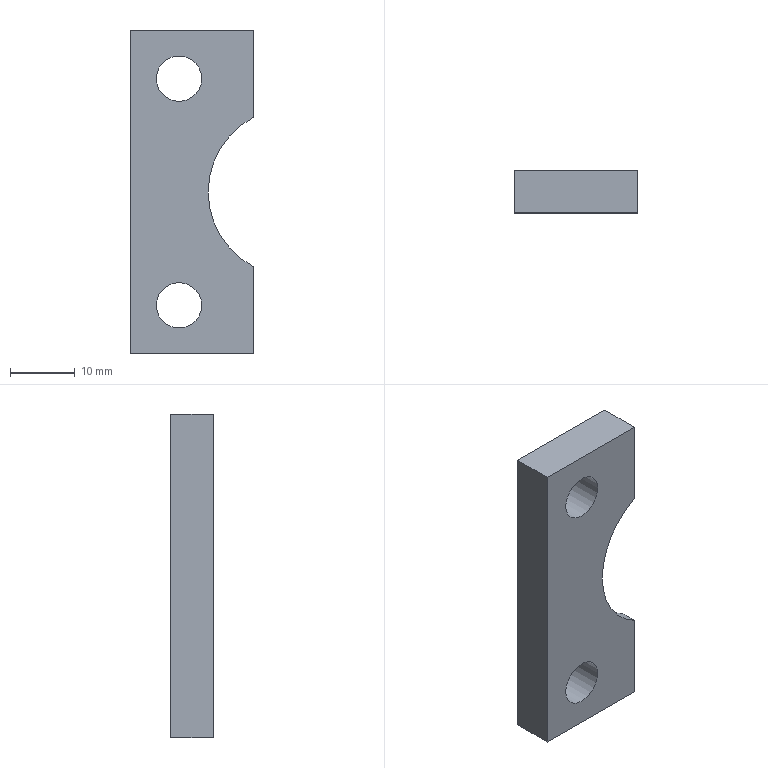Part | NX | features solid 2 | 1 solid | 12 faces | box 19 x 6.5 x 50 mm | volume 4528 mm3 | plane 8 | cylinder 4 | commonest cylinder face diameters 7 x2 26 x1 32 x1
STEP:
#1=CARTESIAN_POINT('',(694.,845.,-199.832));
#2=VERTEX_POINT('',#1);
#3=CARTESIAN_POINT('',(694.,849.,-199.832));
#4=VERTEX_POINT('',#3);
#5=CARTESIAN_POINT('',(694.,842.5,-199.832));
#6=DIRECTION('',(0.,1.,0.));
#7=VECTOR('',#6,1000.);
#8=LINE('',#5,#7);
#9=EDGE_CURVE('',#2,#4,#8,.T.);
#10=ORIENTED_EDGE('',*,*,#9,.T.);
#11=CARTESIAN_POINT('',(694.,849.,-170.168));
#12=VERTEX_POINT('',#11);
#13=CARTESIAN_POINT('',(700.,849.,-185.));
#14=DIRECTION('',(0.,1.,0.));
#15=DIRECTION('',(-1.,0.,0.));
#16=AXIS2_PLACEMENT_3D('',#13,#14,#15);
#17=CIRCLE('',#16,16.);
#18=EDGE_CURVE('',#4,#12,#17,.T.);
#19=ORIENTED_EDGE('',*,*,#18,.T.);
#20=CARTESIAN_POINT('',(694.,845.,-170.168));
#21=VERTEX_POINT('',#20);
#22=CARTESIAN_POINT('',(694.,842.5,-170.168));
#23=DIRECTION('',(0.,1.,0.));
#24=VECTOR('',#23,1000.);
#25=LINE('',#22,#24);
#26=EDGE_CURVE('',#21,#12,#25,.T.);
#27=ORIENTED_EDGE('',*,*,#26,.F.);
#28=CARTESIAN_POINT('',(700.,845.,-185.));
#29=DIRECTION('',(0.,1.,0.));
#30=DIRECTION('',(-1.,0.,0.));
#31=AXIS2_PLACEMENT_3D('',#28,#29,#30);
#32=CIRCLE('',#31,16.);
#33=EDGE_CURVE('',#2,#21,#32,.T.);
#34=ORIENTED_EDGE('',*,*,#33,.F.);
#35=EDGE_LOOP('',(#10,#19,#27,#34));
#36=FACE_BOUND('',#35,.T.);
#37=CARTESIAN_POINT('',(700.,842.5,-185.));
#38=DIRECTION('',(0.,1.,0.));
#39=DIRECTION('',(1.,0.,0.));
#40=AXIS2_PLACEMENT_3D('',#37,#38,#39);
#41=CYLINDRICAL_SURFACE('',#40,16.);
#42=ADVANCED_FACE('',(#36),#41,.F.);
#43=CARTESIAN_POINT('',(679.,842.5,-202.5));
#44=VERTEX_POINT('',#43);
#45=CARTESIAN_POINT('',(682.5,842.5,-202.5));
#46=DIRECTION('',(0.,1.,0.));
#47=DIRECTION('',(-1.,0.,0.));
#48=AXIS2_PLACEMENT_3D('',#45,#46,#47);
#49=CIRCLE('',#48,3.5);
#50=EDGE_CURVE('',#44,#44,#49,.T.);
#51=ORIENTED_EDGE('',*,*,#50,.T.);
#52=EDGE_LOOP('',(#51));
#53=FACE_BOUND('',#52,.T.);
#54=CARTESIAN_POINT('',(694.,842.5,-160.));
#55=VERTEX_POINT('',#54);
#56=CARTESIAN_POINT('',(675.,842.5,-160.));
#57=VERTEX_POINT('',#56);
#58=CARTESIAN_POINT('',(694.,842.5,-160.));
#59=DIRECTION('',(-1.,0.,0.));
#60=VECTOR('',#59,1000.);
#61=LINE('',#58,#60);
#62=EDGE_CURVE('',#55,#57,#61,.T.);
#63=ORIENTED_EDGE('',*,*,#62,.T.);
#64=CARTESIAN_POINT('',(675.,842.5,-210.));
#65=VERTEX_POINT('',#64);
#66=CARTESIAN_POINT('',(675.,842.5,-210.));
#67=DIRECTION('',(0.,0.,1.));
#68=VECTOR('',#67,1000.);
#69=LINE('',#66,#68);
#70=EDGE_CURVE('',#65,#57,#69,.T.);
#71=ORIENTED_EDGE('',*,*,#70,.F.);
#72=CARTESIAN_POINT('',(694.,842.5,-210.));
#73=VERTEX_POINT('',#72);
#74=CARTESIAN_POINT('',(694.,842.5,-210.));
#75=DIRECTION('',(-1.,0.,0.));
#76=VECTOR('',#75,1000.);
#77=LINE('',#74,#76);
#78=EDGE_CURVE('',#73,#65,#77,.T.);
#79=ORIENTED_EDGE('',*,*,#78,.F.);
#80=CARTESIAN_POINT('',(694.,842.5,-196.533));
#81=VERTEX_POINT('',#80);
#82=CARTESIAN_POINT('',(694.,842.5,-196.533));
#83=DIRECTION('',(0.,0.,-1.));
#84=VECTOR('',#83,1000.);
#85=LINE('',#82,#84);
#86=EDGE_CURVE('',#81,#73,#85,.T.);
#87=ORIENTED_EDGE('',*,*,#86,.F.);
#88=CARTESIAN_POINT('',(694.,842.5,-173.467));
#89=VERTEX_POINT('',#88);
#90=CARTESIAN_POINT('',(700.,842.5,-185.));
#91=DIRECTION('',(0.,1.,0.));
#92=DIRECTION('',(-1.,0.,0.));
#93=AXIS2_PLACEMENT_3D('',#90,#91,#92);
#94=CIRCLE('',#93,13.);
#95=EDGE_CURVE('',#81,#89,#94,.T.);
#96=ORIENTED_EDGE('',*,*,#95,.T.);
#97=CARTESIAN_POINT('',(694.,842.5,-160.));
#98=DIRECTION('',(0.,0.,-1.));
#99=VECTOR('',#98,1000.);
#100=LINE('',#97,#99);
#101=EDGE_CURVE('',#55,#89,#100,.T.);
#102=ORIENTED_EDGE('',*,*,#101,.F.);
#103=EDGE_LOOP('',(#63,#71,#79,#87,#96,#102));
#104=FACE_BOUND('',#103,.T.);
#105=CARTESIAN_POINT('',(679.,842.5,-167.5));
#106=VERTEX_POINT('',#105);
#107=CARTESIAN_POINT('',(682.5,842.5,-167.5));
#108=DIRECTION('',(0.,1.,0.));
#109=DIRECTION('',(-1.,0.,0.));
#110=AXIS2_PLACEMENT_3D('',#107,#108,#109);
#111=CIRCLE('',#110,3.5);
#112=EDGE_CURVE('',#106,#106,#111,.T.);
#113=ORIENTED_EDGE('',*,*,#112,.T.);
#114=EDGE_LOOP('',(#113));
#115=FACE_BOUND('',#114,.T.);
#116=CARTESIAN_POINT('',(687.667,842.5,-189.394));
#117=DIRECTION('',(0.,-1.,0.));
#118=DIRECTION('',(-1.,0.,0.));
#119=AXIS2_PLACEMENT_3D('',#116,#117,#118);
#120=PLANE('',#119);
#121=ADVANCED_FACE('',(#53,#104,#115),#120,.T.);
#122=CARTESIAN_POINT('',(679.,849.,-202.5));
#123=VERTEX_POINT('',#122);
#124=CARTESIAN_POINT('',(682.5,849.,-202.5));
#125=DIRECTION('',(0.,1.,0.));
#126=DIRECTION('',(-1.,0.,0.));
#127=AXIS2_PLACEMENT_3D('',#124,#125,#126);
#128=CIRCLE('',#127,3.5);
#129=EDGE_CURVE('',#123,#123,#128,.T.);
#130=ORIENTED_EDGE('',*,*,#129,.F.);
#131=EDGE_LOOP('',(#130));
#132=FACE_BOUND('',#131,.T.);
#133=CARTESIAN_POINT('',(694.,849.,-160.));
#134=VERTEX_POINT('',#133);
#135=CARTESIAN_POINT('',(675.,849.,-160.));
#136=VERTEX_POINT('',#135);
#137=CARTESIAN_POINT('',(694.,849.,-160.));
#138=DIRECTION('',(-1.,0.,0.));
#139=VECTOR('',#138,1000.);
#140=LINE('',#137,#139);
#141=EDGE_CURVE('',#134,#136,#140,.T.);
#142=ORIENTED_EDGE('',*,*,#141,.F.);
#143=CARTESIAN_POINT('',(694.,849.,-160.));
#144=DIRECTION('',(0.,0.,-1.));
#145=VECTOR('',#144,1000.);
#146=LINE('',#143,#145);
#147=EDGE_CURVE('',#134,#12,#146,.T.);
#148=ORIENTED_EDGE('',*,*,#147,.T.);
#149=ORIENTED_EDGE('',*,*,#18,.F.);
#150=CARTESIAN_POINT('',(694.,849.,-210.));
#151=VERTEX_POINT('',#150);
#152=CARTESIAN_POINT('',(694.,849.,-196.533));
#153=DIRECTION('',(0.,0.,-1.));
#154=VECTOR('',#153,1000.);
#155=LINE('',#152,#154);
#156=EDGE_CURVE('',#4,#151,#155,.T.);
#157=ORIENTED_EDGE('',*,*,#156,.T.);
#158=CARTESIAN_POINT('',(675.,849.,-210.));
#159=VERTEX_POINT('',#158);
#160=CARTESIAN_POINT('',(694.,849.,-210.));
#161=DIRECTION('',(-1.,0.,0.));
#162=VECTOR('',#161,1000.);
#163=LINE('',#160,#162);
#164=EDGE_CURVE('',#151,#159,#163,.T.);
#165=ORIENTED_EDGE('',*,*,#164,.T.);
#166=CARTESIAN_POINT('',(675.,849.,-210.));
#167=DIRECTION('',(0.,0.,1.));
#168=VECTOR('',#167,1000.);
#169=LINE('',#166,#168);
#170=EDGE_CURVE('',#159,#136,#169,.T.);
#171=ORIENTED_EDGE('',*,*,#170,.T.);
#172=EDGE_LOOP('',(#142,#148,#149,#157,#165,#171));
#173=FACE_BOUND('',#172,.T.);
#174=CARTESIAN_POINT('',(679.,849.,-167.5));
#175=VERTEX_POINT('',#174);
#176=CARTESIAN_POINT('',(682.5,849.,-167.5));
#177=DIRECTION('',(0.,1.,0.));
#178=DIRECTION('',(-1.,0.,0.));
#179=AXIS2_PLACEMENT_3D('',#176,#177,#178);
#180=CIRCLE('',#179,3.5);
#181=EDGE_CURVE('',#175,#175,#180,.T.);
#182=ORIENTED_EDGE('',*,*,#181,.F.);
#183=EDGE_LOOP('',(#182));
#184=FACE_BOUND('',#183,.T.);
#185=CARTESIAN_POINT('',(687.667,849.,-189.394));
#186=DIRECTION('',(0.,-1.,0.));
#187=DIRECTION('',(-1.,0.,0.));
#188=AXIS2_PLACEMENT_3D('',#185,#186,#187);
#189=PLANE('',#188);
#190=ADVANCED_FACE('',(#132,#173,#184),#189,.F.);
#191=ORIENTED_EDGE('',*,*,#141,.T.);
#192=CARTESIAN_POINT('',(675.,842.5,-160.));
#193=DIRECTION('',(0.,1.,0.));
#194=VECTOR('',#193,1000.);
#195=LINE('',#192,#194);
#196=EDGE_CURVE('',#57,#136,#195,.T.);
#197=ORIENTED_EDGE('',*,*,#196,.F.);
#198=ORIENTED_EDGE('',*,*,#62,.F.);
#199=CARTESIAN_POINT('',(694.,842.5,-160.));
#200=DIRECTION('',(0.,1.,0.));
#201=VECTOR('',#200,1000.);
#202=LINE('',#199,#201);
#203=EDGE_CURVE('',#55,#134,#202,.T.);
#204=ORIENTED_EDGE('',*,*,#203,.T.);
#205=EDGE_LOOP('',(#191,#197,#198,#204));
#206=FACE_BOUND('',#205,.T.);
#207=CARTESIAN_POINT('',(694.,842.5,-160.));
#208=DIRECTION('',(0.,0.,1.));
#209=DIRECTION('',(0.,-1.,0.));
#210=AXIS2_PLACEMENT_3D('',#207,#208,#209);
#211=PLANE('',#210);
#212=ADVANCED_FACE('',(#206),#211,.T.);
#213=ORIENTED_EDGE('',*,*,#147,.F.);
#214=ORIENTED_EDGE('',*,*,#203,.F.);
#215=ORIENTED_EDGE('',*,*,#101,.T.);
#216=CARTESIAN_POINT('',(694.,845.,-173.467));
#217=VERTEX_POINT('',#216);
#218=CARTESIAN_POINT('',(694.,842.5,-173.467));
#219=DIRECTION('',(0.,1.,0.));
#220=VECTOR('',#219,1000.);
#221=LINE('',#218,#220);
#222=EDGE_CURVE('',#89,#217,#221,.T.);
#223=ORIENTED_EDGE('',*,*,#222,.T.);
#224=CARTESIAN_POINT('',(694.,845.,-160.));
#225=DIRECTION('',(0.,0.,-1.));
#226=VECTOR('',#225,1000.);
#227=LINE('',#224,#226);
#228=EDGE_CURVE('',#21,#217,#227,.T.);
#229=ORIENTED_EDGE('',*,*,#228,.F.);
#230=ORIENTED_EDGE('',*,*,#26,.T.);
#231=EDGE_LOOP('',(#213,#214,#215,#223,#229,#230));
#232=FACE_BOUND('',#231,.T.);
#233=CARTESIAN_POINT('',(694.,842.5,-160.));
#234=DIRECTION('',(-1.,0.,0.));
#235=DIRECTION('',(0.,1.,0.));
#236=AXIS2_PLACEMENT_3D('',#233,#234,#235);
#237=PLANE('',#236);
#238=ADVANCED_FACE('',(#232),#237,.F.);
#239=ORIENTED_EDGE('',*,*,#156,.F.);
#240=ORIENTED_EDGE('',*,*,#9,.F.);
#241=CARTESIAN_POINT('',(694.,845.,-196.533));
#242=VERTEX_POINT('',#241);
#243=CARTESIAN_POINT('',(694.,845.,-196.533));
#244=DIRECTION('',(0.,0.,-1.));
#245=VECTOR('',#244,1000.);
#246=LINE('',#243,#245);
#247=EDGE_CURVE('',#242,#2,#246,.T.);
#248=ORIENTED_EDGE('',*,*,#247,.F.);
#249=CARTESIAN_POINT('',(694.,842.5,-196.533));
#250=DIRECTION('',(0.,1.,0.));
#251=VECTOR('',#250,1000.);
#252=LINE('',#249,#251);
#253=EDGE_CURVE('',#81,#242,#252,.T.);
#254=ORIENTED_EDGE('',*,*,#253,.F.);
#255=ORIENTED_EDGE('',*,*,#86,.T.);
#256=CARTESIAN_POINT('',(694.,842.5,-210.));
#257=DIRECTION('',(0.,1.,0.));
#258=VECTOR('',#257,1000.);
#259=LINE('',#256,#258);
#260=EDGE_CURVE('',#73,#151,#259,.T.);
#261=ORIENTED_EDGE('',*,*,#260,.T.);
#262=EDGE_LOOP('',(#239,#240,#248,#254,#255,#261));
#263=FACE_BOUND('',#262,.T.);
#264=CARTESIAN_POINT('',(694.,842.5,-196.533));
#265=DIRECTION('',(-1.,0.,0.));
#266=DIRECTION('',(0.,1.,0.));
#267=AXIS2_PLACEMENT_3D('',#264,#265,#266);
#268=PLANE('',#267);
#269=ADVANCED_FACE('',(#263),#268,.F.);
#270=ORIENTED_EDGE('',*,*,#164,.F.);
#271=ORIENTED_EDGE('',*,*,#260,.F.);
#272=ORIENTED_EDGE('',*,*,#78,.T.);
#273=CARTESIAN_POINT('',(675.,842.5,-210.));
#274=DIRECTION('',(0.,1.,0.));
#275=VECTOR('',#274,1000.);
#276=LINE('',#273,#275);
#277=EDGE_CURVE('',#65,#159,#276,.T.);
#278=ORIENTED_EDGE('',*,*,#277,.T.);
#279=EDGE_LOOP('',(#270,#271,#272,#278));
#280=FACE_BOUND('',#279,.T.);
#281=CARTESIAN_POINT('',(694.,842.5,-210.));
#282=DIRECTION('',(0.,0.,1.));
#283=DIRECTION('',(0.,-1.,0.));
#284=AXIS2_PLACEMENT_3D('',#281,#282,#283);
#285=PLANE('',#284);
#286=ADVANCED_FACE('',(#280),#285,.F.);
#287=ORIENTED_EDGE('',*,*,#170,.F.);
#288=ORIENTED_EDGE('',*,*,#277,.F.);
#289=ORIENTED_EDGE('',*,*,#70,.T.);
#290=ORIENTED_EDGE('',*,*,#196,.T.);
#291=EDGE_LOOP('',(#287,#288,#289,#290));
#292=FACE_BOUND('',#291,.T.);
#293=CARTESIAN_POINT('',(675.,842.5,-210.));
#294=DIRECTION('',(1.,0.,0.));
#295=DIRECTION('',(0.,-1.,0.));
#296=AXIS2_PLACEMENT_3D('',#293,#294,#295);
#297=PLANE('',#296);
#298=ADVANCED_FACE('',(#292),#297,.F.);
#299=ORIENTED_EDGE('',*,*,#50,.F.);
#300=EDGE_LOOP('',(#299));
#301=FACE_BOUND('',#300,.T.);
#302=ORIENTED_EDGE('',*,*,#129,.T.);
#303=EDGE_LOOP('',(#302));
#304=FACE_BOUND('',#303,.T.);
#305=CARTESIAN_POINT('',(682.5,842.5,-202.5));
#306=DIRECTION('',(0.,1.,0.));
#307=DIRECTION('',(1.,0.,0.));
#308=AXIS2_PLACEMENT_3D('',#305,#306,#307);
#309=CYLINDRICAL_SURFACE('',#308,3.5);
#310=ADVANCED_FACE('',(#301,#304),#309,.F.);
#311=ORIENTED_EDGE('',*,*,#112,.F.);
#312=EDGE_LOOP('',(#311));
#313=FACE_BOUND('',#312,.T.);
#314=ORIENTED_EDGE('',*,*,#181,.T.);
#315=EDGE_LOOP('',(#314));
#316=FACE_BOUND('',#315,.T.);
#317=CARTESIAN_POINT('',(682.5,842.5,-167.5));
#318=DIRECTION('',(0.,1.,0.));
#319=DIRECTION('',(1.,0.,0.));
#320=AXIS2_PLACEMENT_3D('',#317,#318,#319);
#321=CYLINDRICAL_SURFACE('',#320,3.5);
#322=ADVANCED_FACE('',(#313,#316),#321,.F.);
#323=CARTESIAN_POINT('',(700.,845.,-185.));
#324=DIRECTION('',(0.,1.,0.));
#325=DIRECTION('',(-1.,0.,0.));
#326=AXIS2_PLACEMENT_3D('',#323,#324,#325);
#327=CIRCLE('',#326,13.);
#328=EDGE_CURVE('',#242,#217,#327,.T.);
#329=ORIENTED_EDGE('',*,*,#328,.T.);
#330=ORIENTED_EDGE('',*,*,#222,.F.);
#331=ORIENTED_EDGE('',*,*,#95,.F.);
#332=ORIENTED_EDGE('',*,*,#253,.T.);
#333=EDGE_LOOP('',(#329,#330,#331,#332));
#334=FACE_BOUND('',#333,.T.);
#335=CARTESIAN_POINT('',(700.,842.5,-185.));
#336=DIRECTION('',(0.,1.,0.));
#337=DIRECTION('',(1.,0.,0.));
#338=AXIS2_PLACEMENT_3D('',#335,#336,#337);
#339=CYLINDRICAL_SURFACE('',#338,13.);
#340=ADVANCED_FACE('',(#334),#339,.F.);
#341=ORIENTED_EDGE('',*,*,#328,.F.);
#342=ORIENTED_EDGE('',*,*,#247,.T.);
#343=ORIENTED_EDGE('',*,*,#33,.T.);
#344=ORIENTED_EDGE('',*,*,#228,.T.);
#345=EDGE_LOOP('',(#341,#342,#343,#344));
#346=FACE_BOUND('',#345,.T.);
#347=CARTESIAN_POINT('',(694.,845.,-188.224));
#348=DIRECTION('',(0.,-1.,0.));
#349=DIRECTION('',(-1.,0.,0.));
#350=AXIS2_PLACEMENT_3D('',#347,#348,#349);
#351=PLANE('',#350);
#352=ADVANCED_FACE('',(#346),#351,.F.);
#353=CLOSED_SHELL('',(#42,#121,#190,#212,#238,#269,#286,#298,#310,#322,#340,#352));
#354=MANIFOLD_SOLID_BREP('',#353);
#355=(LENGTH_UNIT()NAMED_UNIT(*)SI_UNIT(.MILLI.,.METRE.));
#356=UNCERTAINTY_MEASURE_WITH_UNIT(LENGTH_MEASURE(0.00001),#355,'','');
#357=(NAMED_UNIT(*)PLANE_ANGLE_UNIT()SI_UNIT($,.RADIAN.));
#358=(NAMED_UNIT(*)SI_UNIT($,.STERADIAN.)SOLID_ANGLE_UNIT());
#359=(GEOMETRIC_REPRESENTATION_CONTEXT(3)GLOBAL_UNCERTAINTY_ASSIGNED_CONTEXT((#356))GLOBAL_UNIT_ASSIGNED_CONTEXT((#355,#357,#358))REPRESENTATION_CONTEXT('',''));
#360=ADVANCED_BREP_SHAPE_REPRESENTATION('',(#354),#359);